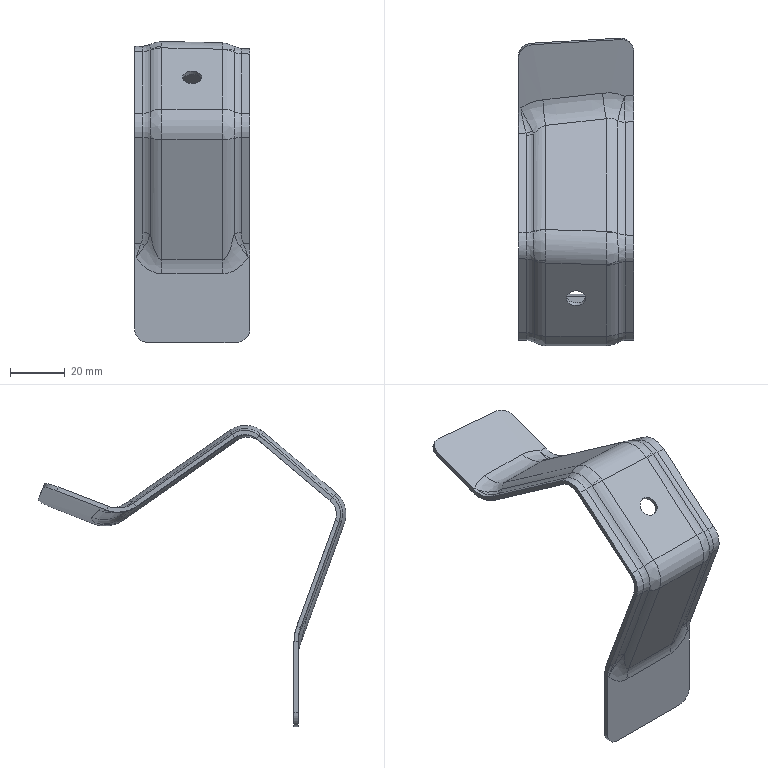Part | STEP file | FNA5401791 | 1 solid | 144 faces | box 42.218 x 112.188 x 109.748 mm | volume 13572 mm3 | spline 79 | cylinder 46 | plane 11 | other 4 | torus 4 | commonest cylinder face diameters 13 x16 16 x10 10 x8 30 x3 33 x3 7 x2